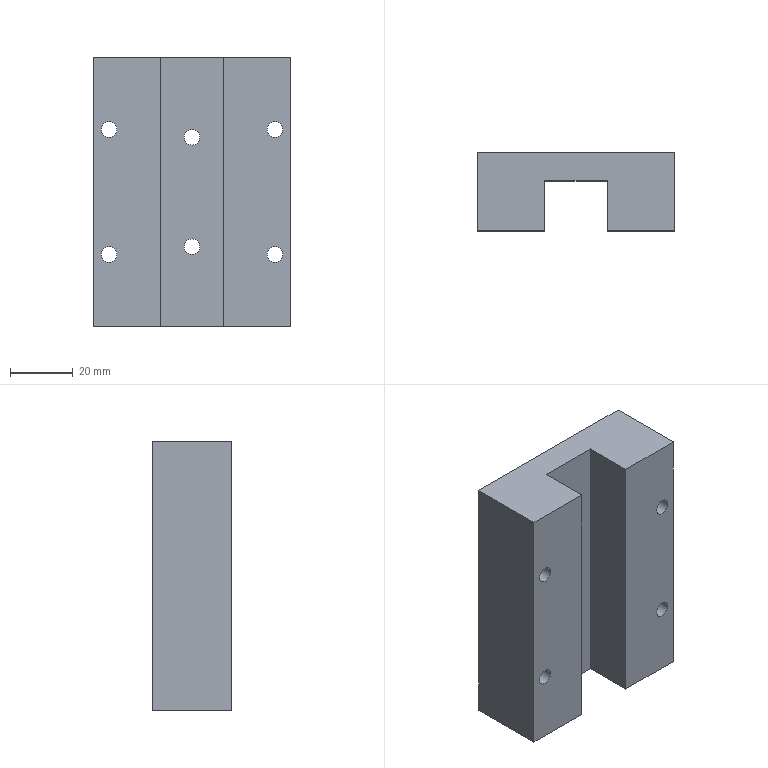Part | NX | 1 solid | 16 faces | box 63 x 25 x 86 mm | volume 105613 mm3 | plane 10 | cylinder 6 | commonest cylinder face diameters 5 x6
STEP:
#1=CARTESIAN_POINT('',(0.,3.5,63.));
#2=VERTEX_POINT('',#1);
#3=CARTESIAN_POINT('',(0.,3.5,60.5));
#4=DIRECTION('',(0.,1.,0.));
#5=DIRECTION('',(0.,0.,1.));
#6=AXIS2_PLACEMENT_3D('',#3,#4,#5);
#7=CIRCLE('',#6,2.5);
#8=EDGE_CURVE('',#2,#2,#7,.T.);
#9=ORIENTED_EDGE('',*,*,#8,.T.);
#10=EDGE_LOOP('',(#9));
#11=FACE_BOUND('',#10,.T.);
#12=CARTESIAN_POINT('',(-10.,3.5,0.));
#13=VERTEX_POINT('',#12);
#14=CARTESIAN_POINT('',(10.,3.5,0.));
#15=VERTEX_POINT('',#14);
#16=CARTESIAN_POINT('',(-10.,3.5,0.));
#17=DIRECTION('',(1.,0.,0.));
#18=VECTOR('',#17,1.);
#19=LINE('',#16,#18);
#20=EDGE_CURVE('',#13,#15,#19,.T.);
#21=ORIENTED_EDGE('',*,*,#20,.T.);
#22=CARTESIAN_POINT('',(10.,3.5,86.));
#23=VERTEX_POINT('',#22);
#24=CARTESIAN_POINT('',(10.,3.5,86.));
#25=DIRECTION('',(0.,0.,-1.));
#26=VECTOR('',#25,1.);
#27=LINE('',#24,#26);
#28=EDGE_CURVE('',#23,#15,#27,.T.);
#29=ORIENTED_EDGE('',*,*,#28,.F.);
#30=CARTESIAN_POINT('',(-10.,3.5,86.));
#31=VERTEX_POINT('',#30);
#32=CARTESIAN_POINT('',(-10.,3.5,86.));
#33=DIRECTION('',(1.,0.,0.));
#34=VECTOR('',#33,1.);
#35=LINE('',#32,#34);
#36=EDGE_CURVE('',#31,#23,#35,.T.);
#37=ORIENTED_EDGE('',*,*,#36,.F.);
#38=CARTESIAN_POINT('',(-10.,3.5,86.));
#39=DIRECTION('',(0.,0.,-1.));
#40=VECTOR('',#39,1.);
#41=LINE('',#38,#40);
#42=EDGE_CURVE('',#31,#13,#41,.T.);
#43=ORIENTED_EDGE('',*,*,#42,.T.);
#44=EDGE_LOOP('',(#21,#29,#37,#43));
#45=FACE_BOUND('',#44,.T.);
#46=CARTESIAN_POINT('',(0.,3.5,28.));
#47=VERTEX_POINT('',#46);
#48=CARTESIAN_POINT('',(0.,3.5,25.5));
#49=DIRECTION('',(0.,-1.,0.));
#50=DIRECTION('',(0.,0.,1.));
#51=AXIS2_PLACEMENT_3D('',#48,#49,#50);
#52=CIRCLE('',#51,2.5);
#53=EDGE_CURVE('',#47,#47,#52,.T.);
#54=ORIENTED_EDGE('',*,*,#53,.F.);
#55=EDGE_LOOP('',(#54));
#56=FACE_BOUND('',#55,.T.);
#57=CARTESIAN_POINT('',(-10.,3.5,86.));
#58=DIRECTION('',(0.,1.,0.));
#59=DIRECTION('',(0.,0.,-1.));
#60=AXIS2_PLACEMENT_3D('',#57,#58,#59);
#61=PLANE('',#60);
#62=ADVANCED_FACE('',(#11,#45,#56),#61,.F.);
#63=CARTESIAN_POINT('',(26.5,-12.5,65.5));
#64=VERTEX_POINT('',#63);
#65=CARTESIAN_POINT('',(26.5,-12.5,63.));
#66=DIRECTION('',(0.,1.,0.));
#67=DIRECTION('',(0.,0.,1.));
#68=AXIS2_PLACEMENT_3D('',#65,#66,#67);
#69=CIRCLE('',#68,2.5);
#70=EDGE_CURVE('',#64,#64,#69,.T.);
#71=ORIENTED_EDGE('',*,*,#70,.T.);
#72=EDGE_LOOP('',(#71));
#73=FACE_BOUND('',#72,.T.);
#74=CARTESIAN_POINT('',(10.,-12.5,0.));
#75=VERTEX_POINT('',#74);
#76=CARTESIAN_POINT('',(31.5,-12.5,0.));
#77=VERTEX_POINT('',#76);
#78=CARTESIAN_POINT('',(10.,-12.5,0.));
#79=DIRECTION('',(1.,0.,0.));
#80=VECTOR('',#79,1.);
#81=LINE('',#78,#80);
#82=EDGE_CURVE('',#75,#77,#81,.T.);
#83=ORIENTED_EDGE('',*,*,#82,.T.);
#84=CARTESIAN_POINT('',(31.5,-12.5,86.));
#85=VERTEX_POINT('',#84);
#86=CARTESIAN_POINT('',(31.5,-12.5,86.));
#87=DIRECTION('',(0.,0.,-1.));
#88=VECTOR('',#87,1.);
#89=LINE('',#86,#88);
#90=EDGE_CURVE('',#85,#77,#89,.T.);
#91=ORIENTED_EDGE('',*,*,#90,.F.);
#92=CARTESIAN_POINT('',(10.,-12.5,86.));
#93=VERTEX_POINT('',#92);
#94=CARTESIAN_POINT('',(10.,-12.5,86.));
#95=DIRECTION('',(1.,0.,0.));
#96=VECTOR('',#95,1.);
#97=LINE('',#94,#96);
#98=EDGE_CURVE('',#93,#85,#97,.T.);
#99=ORIENTED_EDGE('',*,*,#98,.F.);
#100=CARTESIAN_POINT('',(10.,-12.5,86.));
#101=DIRECTION('',(0.,0.,-1.));
#102=VECTOR('',#101,1.);
#103=LINE('',#100,#102);
#104=EDGE_CURVE('',#93,#75,#103,.T.);
#105=ORIENTED_EDGE('',*,*,#104,.T.);
#106=EDGE_LOOP('',(#83,#91,#99,#105));
#107=FACE_BOUND('',#106,.T.);
#108=CARTESIAN_POINT('',(26.5,-12.5,25.5));
#109=VERTEX_POINT('',#108);
#110=CARTESIAN_POINT('',(26.5,-12.5,23.));
#111=DIRECTION('',(0.,-1.,0.));
#112=DIRECTION('',(0.,0.,1.));
#113=AXIS2_PLACEMENT_3D('',#110,#111,#112);
#114=CIRCLE('',#113,2.5);
#115=EDGE_CURVE('',#109,#109,#114,.T.);
#116=ORIENTED_EDGE('',*,*,#115,.F.);
#117=EDGE_LOOP('',(#116));
#118=FACE_BOUND('',#117,.T.);
#119=CARTESIAN_POINT('',(10.,-12.5,86.));
#120=DIRECTION('',(0.,1.,0.));
#121=DIRECTION('',(0.,0.,-1.));
#122=AXIS2_PLACEMENT_3D('',#119,#120,#121);
#123=PLANE('',#122);
#124=ADVANCED_FACE('',(#73,#107,#118),#123,.F.);
#125=CARTESIAN_POINT('',(-26.5,12.5,25.5));
#126=VERTEX_POINT('',#125);
#127=CARTESIAN_POINT('',(-26.5,12.5,23.));
#128=DIRECTION('',(0.,1.,0.));
#129=DIRECTION('',(0.,0.,1.));
#130=AXIS2_PLACEMENT_3D('',#127,#128,#129);
#131=CIRCLE('',#130,2.5);
#132=EDGE_CURVE('',#126,#126,#131,.T.);
#133=ORIENTED_EDGE('',*,*,#132,.F.);
#134=EDGE_LOOP('',(#133));
#135=FACE_BOUND('',#134,.T.);
#136=CARTESIAN_POINT('',(-26.5,12.5,65.5));
#137=VERTEX_POINT('',#136);
#138=CARTESIAN_POINT('',(-26.5,12.5,63.));
#139=DIRECTION('',(0.,1.,0.));
#140=DIRECTION('',(0.,0.,1.));
#141=AXIS2_PLACEMENT_3D('',#138,#139,#140);
#142=CIRCLE('',#141,2.5);
#143=EDGE_CURVE('',#137,#137,#142,.T.);
#144=ORIENTED_EDGE('',*,*,#143,.F.);
#145=EDGE_LOOP('',(#144));
#146=FACE_BOUND('',#145,.T.);
#147=CARTESIAN_POINT('',(0.,12.5,63.));
#148=VERTEX_POINT('',#147);
#149=CARTESIAN_POINT('',(0.,12.5,60.5));
#150=DIRECTION('',(0.,1.,0.));
#151=DIRECTION('',(0.,0.,1.));
#152=AXIS2_PLACEMENT_3D('',#149,#150,#151);
#153=CIRCLE('',#152,2.5);
#154=EDGE_CURVE('',#148,#148,#153,.T.);
#155=ORIENTED_EDGE('',*,*,#154,.F.);
#156=EDGE_LOOP('',(#155));
#157=FACE_BOUND('',#156,.T.);
#158=CARTESIAN_POINT('',(26.5,12.5,65.5));
#159=VERTEX_POINT('',#158);
#160=CARTESIAN_POINT('',(26.5,12.5,63.));
#161=DIRECTION('',(0.,1.,0.));
#162=DIRECTION('',(0.,0.,1.));
#163=AXIS2_PLACEMENT_3D('',#160,#161,#162);
#164=CIRCLE('',#163,2.5);
#165=EDGE_CURVE('',#159,#159,#164,.T.);
#166=ORIENTED_EDGE('',*,*,#165,.F.);
#167=EDGE_LOOP('',(#166));
#168=FACE_BOUND('',#167,.T.);
#169=CARTESIAN_POINT('',(31.5,12.5,0.));
#170=VERTEX_POINT('',#169);
#171=CARTESIAN_POINT('',(-31.5,12.5,0.));
#172=VERTEX_POINT('',#171);
#173=CARTESIAN_POINT('',(31.5,12.5,0.));
#174=DIRECTION('',(-1.,0.,0.));
#175=VECTOR('',#174,1.);
#176=LINE('',#173,#175);
#177=EDGE_CURVE('',#170,#172,#176,.T.);
#178=ORIENTED_EDGE('',*,*,#177,.T.);
#179=CARTESIAN_POINT('',(-31.5,12.5,86.));
#180=VERTEX_POINT('',#179);
#181=CARTESIAN_POINT('',(-31.5,12.5,86.));
#182=DIRECTION('',(0.,0.,-1.));
#183=VECTOR('',#182,1.);
#184=LINE('',#181,#183);
#185=EDGE_CURVE('',#180,#172,#184,.T.);
#186=ORIENTED_EDGE('',*,*,#185,.F.);
#187=CARTESIAN_POINT('',(31.5,12.5,86.));
#188=VERTEX_POINT('',#187);
#189=CARTESIAN_POINT('',(31.5,12.5,86.));
#190=DIRECTION('',(-1.,0.,0.));
#191=VECTOR('',#190,1.);
#192=LINE('',#189,#191);
#193=EDGE_CURVE('',#188,#180,#192,.T.);
#194=ORIENTED_EDGE('',*,*,#193,.F.);
#195=CARTESIAN_POINT('',(31.5,12.5,86.));
#196=DIRECTION('',(0.,0.,-1.));
#197=VECTOR('',#196,1.);
#198=LINE('',#195,#197);
#199=EDGE_CURVE('',#188,#170,#198,.T.);
#200=ORIENTED_EDGE('',*,*,#199,.T.);
#201=EDGE_LOOP('',(#178,#186,#194,#200));
#202=FACE_BOUND('',#201,.T.);
#203=CARTESIAN_POINT('',(0.,12.5,28.));
#204=VERTEX_POINT('',#203);
#205=CARTESIAN_POINT('',(0.,12.5,25.5));
#206=DIRECTION('',(0.,-1.,0.));
#207=DIRECTION('',(0.,0.,1.));
#208=AXIS2_PLACEMENT_3D('',#205,#206,#207);
#209=CIRCLE('',#208,2.5);
#210=EDGE_CURVE('',#204,#204,#209,.T.);
#211=ORIENTED_EDGE('',*,*,#210,.T.);
#212=EDGE_LOOP('',(#211));
#213=FACE_BOUND('',#212,.T.);
#214=CARTESIAN_POINT('',(26.5,12.5,25.5));
#215=VERTEX_POINT('',#214);
#216=CARTESIAN_POINT('',(26.5,12.5,23.));
#217=DIRECTION('',(0.,-1.,0.));
#218=DIRECTION('',(0.,0.,1.));
#219=AXIS2_PLACEMENT_3D('',#216,#217,#218);
#220=CIRCLE('',#219,2.5);
#221=EDGE_CURVE('',#215,#215,#220,.T.);
#222=ORIENTED_EDGE('',*,*,#221,.T.);
#223=EDGE_LOOP('',(#222));
#224=FACE_BOUND('',#223,.T.);
#225=CARTESIAN_POINT('',(31.5,12.5,86.));
#226=DIRECTION('',(0.,-1.,0.));
#227=DIRECTION('',(0.,0.,1.));
#228=AXIS2_PLACEMENT_3D('',#225,#226,#227);
#229=PLANE('',#228);
#230=ADVANCED_FACE('',(#135,#146,#157,#168,#202,#213,#224),#229,.F.);
#231=CARTESIAN_POINT('',(-31.5,-12.5,0.));
#232=VERTEX_POINT('',#231);
#233=CARTESIAN_POINT('',(-31.5,12.5,0.));
#234=DIRECTION('',(0.,-1.,0.));
#235=VECTOR('',#234,1.);
#236=LINE('',#233,#235);
#237=EDGE_CURVE('',#172,#232,#236,.T.);
#238=ORIENTED_EDGE('',*,*,#237,.T.);
#239=CARTESIAN_POINT('',(-31.5,-12.5,86.));
#240=VERTEX_POINT('',#239);
#241=CARTESIAN_POINT('',(-31.5,-12.5,86.));
#242=DIRECTION('',(0.,0.,-1.));
#243=VECTOR('',#242,1.);
#244=LINE('',#241,#243);
#245=EDGE_CURVE('',#240,#232,#244,.T.);
#246=ORIENTED_EDGE('',*,*,#245,.F.);
#247=CARTESIAN_POINT('',(-31.5,12.5,86.));
#248=DIRECTION('',(0.,-1.,0.));
#249=VECTOR('',#248,1.);
#250=LINE('',#247,#249);
#251=EDGE_CURVE('',#180,#240,#250,.T.);
#252=ORIENTED_EDGE('',*,*,#251,.F.);
#253=ORIENTED_EDGE('',*,*,#185,.T.);
#254=EDGE_LOOP('',(#238,#246,#252,#253));
#255=FACE_OUTER_BOUND('',#254,.T.);
#256=CARTESIAN_POINT('',(-31.5,12.5,86.));
#257=DIRECTION('',(1.,0.,0.));
#258=DIRECTION('',(0.,0.,1.));
#259=AXIS2_PLACEMENT_3D('',#256,#257,#258);
#260=PLANE('',#259);
#261=ADVANCED_FACE('',(#255),#260,.F.);
#262=CARTESIAN_POINT('',(-26.5,-12.5,25.5));
#263=VERTEX_POINT('',#262);
#264=CARTESIAN_POINT('',(-26.5,-12.5,23.));
#265=DIRECTION('',(0.,1.,0.));
#266=DIRECTION('',(0.,0.,1.));
#267=AXIS2_PLACEMENT_3D('',#264,#265,#266);
#268=CIRCLE('',#267,2.5);
#269=EDGE_CURVE('',#263,#263,#268,.T.);
#270=ORIENTED_EDGE('',*,*,#269,.T.);
#271=EDGE_LOOP('',(#270));
#272=FACE_BOUND('',#271,.T.);
#273=CARTESIAN_POINT('',(-26.5,-12.5,65.5));
#274=VERTEX_POINT('',#273);
#275=CARTESIAN_POINT('',(-26.5,-12.5,63.));
#276=DIRECTION('',(0.,1.,0.));
#277=DIRECTION('',(0.,0.,1.));
#278=AXIS2_PLACEMENT_3D('',#275,#276,#277);
#279=CIRCLE('',#278,2.5);
#280=EDGE_CURVE('',#274,#274,#279,.T.);
#281=ORIENTED_EDGE('',*,*,#280,.T.);
#282=EDGE_LOOP('',(#281));
#283=FACE_BOUND('',#282,.T.);
#284=CARTESIAN_POINT('',(-10.,-12.5,0.));
#285=VERTEX_POINT('',#284);
#286=CARTESIAN_POINT('',(-31.5,-12.5,0.));
#287=DIRECTION('',(1.,0.,0.));
#288=VECTOR('',#287,1.);
#289=LINE('',#286,#288);
#290=EDGE_CURVE('',#232,#285,#289,.T.);
#291=ORIENTED_EDGE('',*,*,#290,.T.);
#292=CARTESIAN_POINT('',(-10.,-12.5,86.));
#293=VERTEX_POINT('',#292);
#294=CARTESIAN_POINT('',(-10.,-12.5,86.));
#295=DIRECTION('',(0.,0.,-1.));
#296=VECTOR('',#295,1.);
#297=LINE('',#294,#296);
#298=EDGE_CURVE('',#293,#285,#297,.T.);
#299=ORIENTED_EDGE('',*,*,#298,.F.);
#300=CARTESIAN_POINT('',(-31.5,-12.5,86.));
#301=DIRECTION('',(1.,0.,0.));
#302=VECTOR('',#301,1.);
#303=LINE('',#300,#302);
#304=EDGE_CURVE('',#240,#293,#303,.T.);
#305=ORIENTED_EDGE('',*,*,#304,.F.);
#306=ORIENTED_EDGE('',*,*,#245,.T.);
#307=EDGE_LOOP('',(#291,#299,#305,#306));
#308=FACE_BOUND('',#307,.T.);
#309=CARTESIAN_POINT('',(-31.5,-12.5,86.));
#310=DIRECTION('',(0.,1.,0.));
#311=DIRECTION('',(0.,0.,-1.));
#312=AXIS2_PLACEMENT_3D('',#309,#310,#311);
#313=PLANE('',#312);
#314=ADVANCED_FACE('',(#272,#283,#308),#313,.F.);
#315=CARTESIAN_POINT('',(-10.,-12.5,0.));
#316=DIRECTION('',(0.,1.,0.));
#317=VECTOR('',#316,1.);
#318=LINE('',#315,#317);
#319=EDGE_CURVE('',#285,#13,#318,.T.);
#320=ORIENTED_EDGE('',*,*,#319,.T.);
#321=ORIENTED_EDGE('',*,*,#42,.F.);
#322=CARTESIAN_POINT('',(-10.,-12.5,86.));
#323=DIRECTION('',(0.,1.,0.));
#324=VECTOR('',#323,1.);
#325=LINE('',#322,#324);
#326=EDGE_CURVE('',#293,#31,#325,.T.);
#327=ORIENTED_EDGE('',*,*,#326,.F.);
#328=ORIENTED_EDGE('',*,*,#298,.T.);
#329=EDGE_LOOP('',(#320,#321,#327,#328));
#330=FACE_OUTER_BOUND('',#329,.T.);
#331=CARTESIAN_POINT('',(-10.,-12.5,86.));
#332=DIRECTION('',(-1.,0.,0.));
#333=DIRECTION('',(0.,0.,-1.));
#334=AXIS2_PLACEMENT_3D('',#331,#332,#333);
#335=PLANE('',#334);
#336=ADVANCED_FACE('',(#330),#335,.F.);
#337=CARTESIAN_POINT('',(10.,3.5,0.));
#338=DIRECTION('',(0.,-1.,0.));
#339=VECTOR('',#338,1.);
#340=LINE('',#337,#339);
#341=EDGE_CURVE('',#15,#75,#340,.T.);
#342=ORIENTED_EDGE('',*,*,#341,.T.);
#343=ORIENTED_EDGE('',*,*,#104,.F.);
#344=CARTESIAN_POINT('',(10.,3.5,86.));
#345=DIRECTION('',(0.,-1.,0.));
#346=VECTOR('',#345,1.);
#347=LINE('',#344,#346);
#348=EDGE_CURVE('',#23,#93,#347,.T.);
#349=ORIENTED_EDGE('',*,*,#348,.F.);
#350=ORIENTED_EDGE('',*,*,#28,.T.);
#351=EDGE_LOOP('',(#342,#343,#349,#350));
#352=FACE_OUTER_BOUND('',#351,.T.);
#353=CARTESIAN_POINT('',(10.,3.5,86.));
#354=DIRECTION('',(1.,0.,0.));
#355=DIRECTION('',(0.,0.,1.));
#356=AXIS2_PLACEMENT_3D('',#353,#354,#355);
#357=PLANE('',#356);
#358=ADVANCED_FACE('',(#352),#357,.F.);
#359=CARTESIAN_POINT('',(31.5,-12.5,0.));
#360=DIRECTION('',(0.,1.,0.));
#361=VECTOR('',#360,1.);
#362=LINE('',#359,#361);
#363=EDGE_CURVE('',#77,#170,#362,.T.);
#364=ORIENTED_EDGE('',*,*,#363,.T.);
#365=ORIENTED_EDGE('',*,*,#199,.F.);
#366=CARTESIAN_POINT('',(31.5,-12.5,86.));
#367=DIRECTION('',(0.,1.,0.));
#368=VECTOR('',#367,1.);
#369=LINE('',#366,#368);
#370=EDGE_CURVE('',#85,#188,#369,.T.);
#371=ORIENTED_EDGE('',*,*,#370,.F.);
#372=ORIENTED_EDGE('',*,*,#90,.T.);
#373=EDGE_LOOP('',(#364,#365,#371,#372));
#374=FACE_OUTER_BOUND('',#373,.T.);
#375=CARTESIAN_POINT('',(31.5,-12.5,86.));
#376=DIRECTION('',(-1.,0.,0.));
#377=DIRECTION('',(0.,0.,-1.));
#378=AXIS2_PLACEMENT_3D('',#375,#376,#377);
#379=PLANE('',#378);
#380=ADVANCED_FACE('',(#374),#379,.F.);
#381=ORIENTED_EDGE('',*,*,#251,.T.);
#382=ORIENTED_EDGE('',*,*,#304,.T.);
#383=ORIENTED_EDGE('',*,*,#326,.T.);
#384=ORIENTED_EDGE('',*,*,#36,.T.);
#385=ORIENTED_EDGE('',*,*,#348,.T.);
#386=ORIENTED_EDGE('',*,*,#98,.T.);
#387=ORIENTED_EDGE('',*,*,#370,.T.);
#388=ORIENTED_EDGE('',*,*,#193,.T.);
#389=EDGE_LOOP('',(#381,#382,#383,#384,#385,#386,#387,#388));
#390=FACE_OUTER_BOUND('',#389,.T.);
#391=CARTESIAN_POINT('',(0.,0.,86.));
#392=DIRECTION('',(0.,0.,1.));
#393=DIRECTION('',(-1.,0.,0.));
#394=AXIS2_PLACEMENT_3D('',#391,#392,#393);
#395=PLANE('',#394);
#396=ADVANCED_FACE('',(#390),#395,.T.);
#397=ORIENTED_EDGE('',*,*,#237,.F.);
#398=ORIENTED_EDGE('',*,*,#177,.F.);
#399=ORIENTED_EDGE('',*,*,#363,.F.);
#400=ORIENTED_EDGE('',*,*,#82,.F.);
#401=ORIENTED_EDGE('',*,*,#341,.F.);
#402=ORIENTED_EDGE('',*,*,#20,.F.);
#403=ORIENTED_EDGE('',*,*,#319,.F.);
#404=ORIENTED_EDGE('',*,*,#290,.F.);
#405=EDGE_LOOP('',(#397,#398,#399,#400,#401,#402,#403,#404));
#406=FACE_OUTER_BOUND('',#405,.T.);
#407=CARTESIAN_POINT('',(0.,0.,0.));
#408=DIRECTION('',(0.,0.,1.));
#409=DIRECTION('',(-1.,0.,0.));
#410=AXIS2_PLACEMENT_3D('',#407,#408,#409);
#411=PLANE('',#410);
#412=ADVANCED_FACE('',(#406),#411,.F.);
#413=ORIENTED_EDGE('',*,*,#165,.T.);
#414=EDGE_LOOP('',(#413));
#415=FACE_BOUND('',#414,.T.);
#416=ORIENTED_EDGE('',*,*,#70,.F.);
#417=EDGE_LOOP('',(#416));
#418=FACE_BOUND('',#417,.T.);
#419=CARTESIAN_POINT('',(26.5,-73.5,63.));
#420=DIRECTION('',(0.,1.,0.));
#421=DIRECTION('',(0.,0.,-1.));
#422=AXIS2_PLACEMENT_3D('',#419,#420,#421);
#423=CYLINDRICAL_SURFACE('',#422,2.5);
#424=ADVANCED_FACE('',(#415,#418),#423,.F.);
#425=ORIENTED_EDGE('',*,*,#154,.T.);
#426=EDGE_LOOP('',(#425));
#427=FACE_BOUND('',#426,.T.);
#428=ORIENTED_EDGE('',*,*,#8,.F.);
#429=EDGE_LOOP('',(#428));
#430=FACE_BOUND('',#429,.T.);
#431=CARTESIAN_POINT('',(0.,-73.5,60.5));
#432=DIRECTION('',(0.,1.,0.));
#433=DIRECTION('',(0.,0.,-1.));
#434=AXIS2_PLACEMENT_3D('',#431,#432,#433);
#435=CYLINDRICAL_SURFACE('',#434,2.5);
#436=ADVANCED_FACE('',(#427,#430),#435,.F.);
#437=ORIENTED_EDGE('',*,*,#143,.T.);
#438=EDGE_LOOP('',(#437));
#439=FACE_BOUND('',#438,.T.);
#440=ORIENTED_EDGE('',*,*,#280,.F.);
#441=EDGE_LOOP('',(#440));
#442=FACE_BOUND('',#441,.T.);
#443=CARTESIAN_POINT('',(-26.5,-73.5,63.));
#444=DIRECTION('',(0.,1.,0.));
#445=DIRECTION('',(0.,0.,-1.));
#446=AXIS2_PLACEMENT_3D('',#443,#444,#445);
#447=CYLINDRICAL_SURFACE('',#446,2.5);
#448=ADVANCED_FACE('',(#439,#442),#447,.F.);
#449=ORIENTED_EDGE('',*,*,#132,.T.);
#450=EDGE_LOOP('',(#449));
#451=FACE_BOUND('',#450,.T.);
#452=ORIENTED_EDGE('',*,*,#269,.F.);
#453=EDGE_LOOP('',(#452));
#454=FACE_BOUND('',#453,.T.);
#455=CARTESIAN_POINT('',(-26.5,-73.5,23.));
#456=DIRECTION('',(0.,1.,0.));
#457=DIRECTION('',(0.,0.,-1.));
#458=AXIS2_PLACEMENT_3D('',#455,#456,#457);
#459=CYLINDRICAL_SURFACE('',#458,2.5);
#460=ADVANCED_FACE('',(#451,#454),#459,.F.);
#461=ORIENTED_EDGE('',*,*,#210,.F.);
#462=EDGE_LOOP('',(#461));
#463=FACE_BOUND('',#462,.T.);
#464=ORIENTED_EDGE('',*,*,#53,.T.);
#465=EDGE_LOOP('',(#464));
#466=FACE_BOUND('',#465,.T.);
#467=CARTESIAN_POINT('',(0.,-73.5,25.5));
#468=DIRECTION('',(0.,1.,0.));
#469=DIRECTION('',(0.,0.,-1.));
#470=AXIS2_PLACEMENT_3D('',#467,#468,#469);
#471=CYLINDRICAL_SURFACE('',#470,2.5);
#472=ADVANCED_FACE('',(#463,#466),#471,.F.);
#473=ORIENTED_EDGE('',*,*,#221,.F.);
#474=EDGE_LOOP('',(#473));
#475=FACE_BOUND('',#474,.T.);
#476=ORIENTED_EDGE('',*,*,#115,.T.);
#477=EDGE_LOOP('',(#476));
#478=FACE_BOUND('',#477,.T.);
#479=CARTESIAN_POINT('',(26.5,-73.5,23.));
#480=DIRECTION('',(0.,1.,0.));
#481=DIRECTION('',(0.,0.,-1.));
#482=AXIS2_PLACEMENT_3D('',#479,#480,#481);
#483=CYLINDRICAL_SURFACE('',#482,2.5);
#484=ADVANCED_FACE('',(#475,#478),#483,.F.);
#485=CLOSED_SHELL('',(#62,#124,#230,#261,#314,#336,#358,#380,#396,#412,#424,#436,#448,#460,#472,#484));
#486=MANIFOLD_SOLID_BREP('',#485);
#487=(LENGTH_UNIT()NAMED_UNIT(*)SI_UNIT(.MILLI.,.METRE.));
#488=UNCERTAINTY_MEASURE_WITH_UNIT(LENGTH_MEASURE(0.00002),#487,'','');
#489=(NAMED_UNIT(*)PLANE_ANGLE_UNIT()SI_UNIT($,.RADIAN.));
#490=PLANE_ANGLE_MEASURE_WITH_UNIT(PLANE_ANGLE_MEASURE(0.01745),#489);
#491=DIMENSIONAL_EXPONENTS(0.,0.,0.,0.,0.,0.,0.);
#492=(CONVERSION_BASED_UNIT('DEGREE',#490)NAMED_UNIT(#491)PLANE_ANGLE_UNIT());
#493=(NAMED_UNIT(*)SI_UNIT($,.STERADIAN.)SOLID_ANGLE_UNIT());
#494=(GEOMETRIC_REPRESENTATION_CONTEXT(3)GLOBAL_UNCERTAINTY_ASSIGNED_CONTEXT((#488))GLOBAL_UNIT_ASSIGNED_CONTEXT((#487,#492,#493))REPRESENTATION_CONTEXT('',''));
#495=ADVANCED_BREP_SHAPE_REPRESENTATION('',(#486),#494);